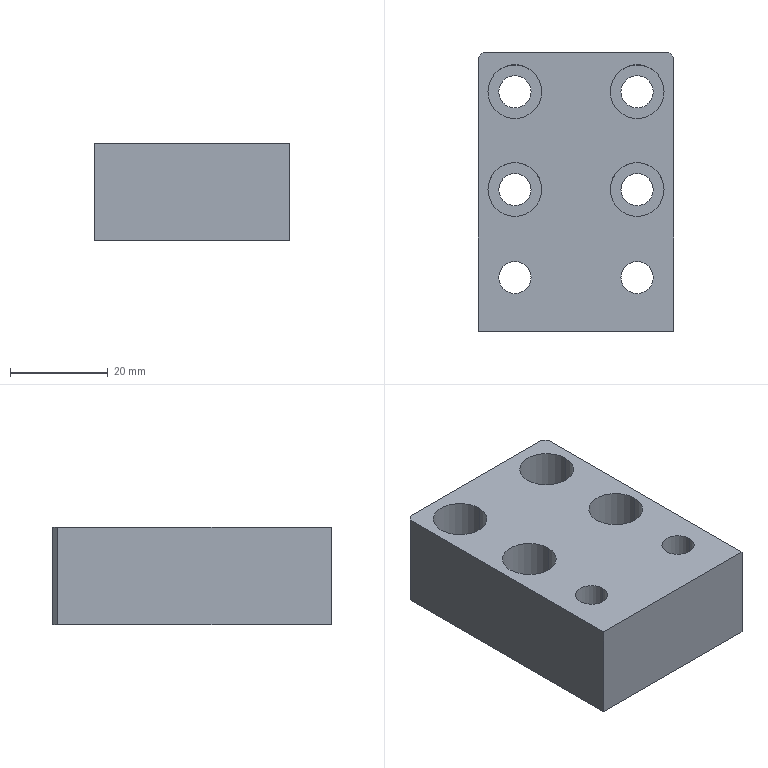Part | SolidWorks | features BaseBody 1 | 1 solid | 38 faces | box 40 x 57 x 20 mm | volume 37168 mm3 | cylinder 24 | plane 14 | commonest cylinder face diameters 6.6 x12 11 x12
STEP:
#1=CARTESIAN_POINT('',(-7.,-17.5,11.8));
#2=VERTEX_POINT('',#1);
#3=CARTESIAN_POINT('',(-18.,-17.5,11.8));
#4=VERTEX_POINT('',#3);
#5=CARTESIAN_POINT('',(-12.5,-17.5,11.8));
#6=DIRECTION('',(0.,0.,-1.));
#7=DIRECTION('',(-1.,0.,0.));
#8=AXIS2_PLACEMENT_3D('',#5,#6,#7);
#9=CIRCLE('',#8,5.5);
#10=EDGE_CURVE('',#2,#4,#9,.T.);
#11=ORIENTED_EDGE('',*,*,#10,.F.);
#12=CARTESIAN_POINT('',(-7.,-17.5,0.));
#13=VERTEX_POINT('',#12);
#14=CARTESIAN_POINT('',(-7.,-17.5,0.));
#15=DIRECTION('',(0.,0.,-1.));
#16=VECTOR('',#15,1000.);
#17=LINE('',#14,#16);
#18=EDGE_CURVE('',#2,#13,#17,.T.);
#19=ORIENTED_EDGE('',*,*,#18,.T.);
#20=CARTESIAN_POINT('',(-18.,-17.5,0.));
#21=VERTEX_POINT('',#20);
#22=CARTESIAN_POINT('',(-12.5,-17.5,0.));
#23=DIRECTION('',(0.,0.,-1.));
#24=DIRECTION('',(-1.,0.,0.));
#25=AXIS2_PLACEMENT_3D('',#22,#23,#24);
#26=CIRCLE('',#25,5.5);
#27=EDGE_CURVE('',#13,#21,#26,.T.);
#28=ORIENTED_EDGE('',*,*,#27,.T.);
#29=CARTESIAN_POINT('',(-18.,-17.5,0.));
#30=DIRECTION('',(0.,0.,-1.));
#31=VECTOR('',#30,1000.);
#32=LINE('',#29,#31);
#33=EDGE_CURVE('',#4,#21,#32,.T.);
#34=ORIENTED_EDGE('',*,*,#33,.F.);
#35=EDGE_LOOP('',(#11,#19,#28,#34));
#36=FACE_OUTER_BOUND('',#35,.T.);
#37=CARTESIAN_POINT('',(-12.5,-17.5,0.));
#38=DIRECTION('',(0.,0.,-1.));
#39=DIRECTION('',(-1.,0.,0.));
#40=AXIS2_PLACEMENT_3D('',#37,#38,#39);
#41=CYLINDRICAL_SURFACE('',#40,5.5);
#42=ADVANCED_FACE('',(#36),#41,.F.);
#43=CARTESIAN_POINT('',(-9.2,-17.5,20.));
#44=VERTEX_POINT('',#43);
#45=CARTESIAN_POINT('',(-15.8,-17.5,20.));
#46=VERTEX_POINT('',#45);
#47=CARTESIAN_POINT('',(-12.5,-17.5,20.));
#48=DIRECTION('',(0.,0.,-1.));
#49=DIRECTION('',(-1.,0.,0.));
#50=AXIS2_PLACEMENT_3D('',#47,#48,#49);
#51=CIRCLE('',#50,3.3);
#52=EDGE_CURVE('',#44,#46,#51,.T.);
#53=ORIENTED_EDGE('',*,*,#52,.F.);
#54=CARTESIAN_POINT('',(-9.2,-17.5,11.8));
#55=VERTEX_POINT('',#54);
#56=CARTESIAN_POINT('',(-9.2,-17.5,0.));
#57=DIRECTION('',(0.,0.,-1.));
#58=VECTOR('',#57,1000.);
#59=LINE('',#56,#58);
#60=EDGE_CURVE('',#44,#55,#59,.T.);
#61=ORIENTED_EDGE('',*,*,#60,.T.);
#62=CARTESIAN_POINT('',(-15.8,-17.5,11.8));
#63=VERTEX_POINT('',#62);
#64=CARTESIAN_POINT('',(-12.5,-17.5,11.8));
#65=DIRECTION('',(0.,0.,-1.));
#66=DIRECTION('',(-1.,0.,0.));
#67=AXIS2_PLACEMENT_3D('',#64,#65,#66);
#68=CIRCLE('',#67,3.3);
#69=EDGE_CURVE('',#55,#63,#68,.T.);
#70=ORIENTED_EDGE('',*,*,#69,.T.);
#71=CARTESIAN_POINT('',(-15.8,-17.5,0.));
#72=DIRECTION('',(0.,0.,-1.));
#73=VECTOR('',#72,1000.);
#74=LINE('',#71,#73);
#75=EDGE_CURVE('',#46,#63,#74,.T.);
#76=ORIENTED_EDGE('',*,*,#75,.F.);
#77=EDGE_LOOP('',(#53,#61,#70,#76));
#78=FACE_OUTER_BOUND('',#77,.T.);
#79=CARTESIAN_POINT('',(-12.5,-17.5,0.));
#80=DIRECTION('',(0.,0.,-1.));
#81=DIRECTION('',(-1.,0.,0.));
#82=AXIS2_PLACEMENT_3D('',#79,#80,#81);
#83=CYLINDRICAL_SURFACE('',#82,3.3);
#84=ADVANCED_FACE('',(#78),#83,.F.);
#85=CARTESIAN_POINT('',(18.,-17.5,11.8));
#86=VERTEX_POINT('',#85);
#87=CARTESIAN_POINT('',(7.,-17.5,11.8));
#88=VERTEX_POINT('',#87);
#89=CARTESIAN_POINT('',(12.5,-17.5,11.8));
#90=DIRECTION('',(0.,0.,-1.));
#91=DIRECTION('',(-1.,0.,0.));
#92=AXIS2_PLACEMENT_3D('',#89,#90,#91);
#93=CIRCLE('',#92,5.5);
#94=EDGE_CURVE('',#86,#88,#93,.T.);
#95=ORIENTED_EDGE('',*,*,#94,.F.);
#96=CARTESIAN_POINT('',(18.,-17.5,0.));
#97=VERTEX_POINT('',#96);
#98=CARTESIAN_POINT('',(18.,-17.5,0.));
#99=DIRECTION('',(0.,0.,-1.));
#100=VECTOR('',#99,1000.);
#101=LINE('',#98,#100);
#102=EDGE_CURVE('',#86,#97,#101,.T.);
#103=ORIENTED_EDGE('',*,*,#102,.T.);
#104=CARTESIAN_POINT('',(7.,-17.5,0.));
#105=VERTEX_POINT('',#104);
#106=CARTESIAN_POINT('',(12.5,-17.5,0.));
#107=DIRECTION('',(0.,0.,-1.));
#108=DIRECTION('',(-1.,0.,0.));
#109=AXIS2_PLACEMENT_3D('',#106,#107,#108);
#110=CIRCLE('',#109,5.5);
#111=EDGE_CURVE('',#97,#105,#110,.T.);
#112=ORIENTED_EDGE('',*,*,#111,.T.);
#113=CARTESIAN_POINT('',(7.,-17.5,0.));
#114=DIRECTION('',(0.,0.,-1.));
#115=VECTOR('',#114,1000.);
#116=LINE('',#113,#115);
#117=EDGE_CURVE('',#88,#105,#116,.T.);
#118=ORIENTED_EDGE('',*,*,#117,.F.);
#119=EDGE_LOOP('',(#95,#103,#112,#118));
#120=FACE_OUTER_BOUND('',#119,.T.);
#121=CARTESIAN_POINT('',(12.5,-17.5,0.));
#122=DIRECTION('',(0.,0.,-1.));
#123=DIRECTION('',(-1.,0.,0.));
#124=AXIS2_PLACEMENT_3D('',#121,#122,#123);
#125=CYLINDRICAL_SURFACE('',#124,5.5);
#126=ADVANCED_FACE('',(#120),#125,.F.);
#127=CARTESIAN_POINT('',(15.8,-17.5,20.));
#128=VERTEX_POINT('',#127);
#129=CARTESIAN_POINT('',(9.2,-17.5,20.));
#130=VERTEX_POINT('',#129);
#131=CARTESIAN_POINT('',(12.5,-17.5,20.));
#132=DIRECTION('',(0.,0.,-1.));
#133=DIRECTION('',(-1.,0.,0.));
#134=AXIS2_PLACEMENT_3D('',#131,#132,#133);
#135=CIRCLE('',#134,3.3);
#136=EDGE_CURVE('',#128,#130,#135,.T.);
#137=ORIENTED_EDGE('',*,*,#136,.F.);
#138=CARTESIAN_POINT('',(15.8,-17.5,11.8));
#139=VERTEX_POINT('',#138);
#140=CARTESIAN_POINT('',(15.8,-17.5,0.));
#141=DIRECTION('',(0.,0.,-1.));
#142=VECTOR('',#141,1000.);
#143=LINE('',#140,#142);
#144=EDGE_CURVE('',#128,#139,#143,.T.);
#145=ORIENTED_EDGE('',*,*,#144,.T.);
#146=CARTESIAN_POINT('',(9.2,-17.5,11.8));
#147=VERTEX_POINT('',#146);
#148=CARTESIAN_POINT('',(12.5,-17.5,11.8));
#149=DIRECTION('',(0.,0.,-1.));
#150=DIRECTION('',(-1.,0.,0.));
#151=AXIS2_PLACEMENT_3D('',#148,#149,#150);
#152=CIRCLE('',#151,3.3);
#153=EDGE_CURVE('',#139,#147,#152,.T.);
#154=ORIENTED_EDGE('',*,*,#153,.T.);
#155=CARTESIAN_POINT('',(9.2,-17.5,0.));
#156=DIRECTION('',(0.,0.,-1.));
#157=VECTOR('',#156,1000.);
#158=LINE('',#155,#157);
#159=EDGE_CURVE('',#130,#147,#158,.T.);
#160=ORIENTED_EDGE('',*,*,#159,.F.);
#161=EDGE_LOOP('',(#137,#145,#154,#160));
#162=FACE_OUTER_BOUND('',#161,.T.);
#163=CARTESIAN_POINT('',(12.5,-17.5,0.));
#164=DIRECTION('',(0.,0.,-1.));
#165=DIRECTION('',(-1.,0.,0.));
#166=AXIS2_PLACEMENT_3D('',#163,#164,#165);
#167=CYLINDRICAL_SURFACE('',#166,3.3);
#168=ADVANCED_FACE('',(#162),#167,.F.);
#169=CARTESIAN_POINT('',(7.,20.5,8.2));
#170=VERTEX_POINT('',#169);
#171=CARTESIAN_POINT('',(18.,20.5,8.2));
#172=VERTEX_POINT('',#171);
#173=CARTESIAN_POINT('',(12.5,20.5,8.2));
#174=DIRECTION('',(0.,0.,1.));
#175=DIRECTION('',(1.,0.,0.));
#176=AXIS2_PLACEMENT_3D('',#173,#174,#175);
#177=CIRCLE('',#176,5.5);
#178=EDGE_CURVE('',#170,#172,#177,.T.);
#179=ORIENTED_EDGE('',*,*,#178,.F.);
#180=CARTESIAN_POINT('',(7.,20.5,20.));
#181=VERTEX_POINT('',#180);
#182=CARTESIAN_POINT('',(7.,20.5,20.));
#183=DIRECTION('',(0.,0.,1.));
#184=VECTOR('',#183,1000.);
#185=LINE('',#182,#184);
#186=EDGE_CURVE('',#170,#181,#185,.T.);
#187=ORIENTED_EDGE('',*,*,#186,.T.);
#188=CARTESIAN_POINT('',(18.,20.5,20.));
#189=VERTEX_POINT('',#188);
#190=CARTESIAN_POINT('',(12.5,20.5,20.));
#191=DIRECTION('',(0.,0.,1.));
#192=DIRECTION('',(1.,0.,0.));
#193=AXIS2_PLACEMENT_3D('',#190,#191,#192);
#194=CIRCLE('',#193,5.5);
#195=EDGE_CURVE('',#181,#189,#194,.T.);
#196=ORIENTED_EDGE('',*,*,#195,.T.);
#197=CARTESIAN_POINT('',(18.,20.5,20.));
#198=DIRECTION('',(0.,0.,1.));
#199=VECTOR('',#198,1000.);
#200=LINE('',#197,#199);
#201=EDGE_CURVE('',#172,#189,#200,.T.);
#202=ORIENTED_EDGE('',*,*,#201,.F.);
#203=EDGE_LOOP('',(#179,#187,#196,#202));
#204=FACE_OUTER_BOUND('',#203,.T.);
#205=CARTESIAN_POINT('',(12.5,20.5,20.));
#206=DIRECTION('',(0.,0.,1.));
#207=DIRECTION('',(1.,0.,0.));
#208=AXIS2_PLACEMENT_3D('',#205,#206,#207);
#209=CYLINDRICAL_SURFACE('',#208,5.5);
#210=ADVANCED_FACE('',(#204),#209,.F.);
#211=CARTESIAN_POINT('',(15.8,20.5,0.));
#212=VERTEX_POINT('',#211);
#213=CARTESIAN_POINT('',(9.2,20.5,0.));
#214=VERTEX_POINT('',#213);
#215=CARTESIAN_POINT('',(12.5,20.5,0.));
#216=DIRECTION('',(0.,0.,-1.));
#217=DIRECTION('',(-1.,0.,0.));
#218=AXIS2_PLACEMENT_3D('',#215,#216,#217);
#219=CIRCLE('',#218,3.3);
#220=EDGE_CURVE('',#212,#214,#219,.T.);
#221=ORIENTED_EDGE('',*,*,#220,.T.);
#222=CARTESIAN_POINT('',(9.2,20.5,8.2));
#223=VERTEX_POINT('',#222);
#224=CARTESIAN_POINT('',(9.2,20.5,20.));
#225=DIRECTION('',(0.,0.,1.));
#226=VECTOR('',#225,1000.);
#227=LINE('',#224,#226);
#228=EDGE_CURVE('',#214,#223,#227,.T.);
#229=ORIENTED_EDGE('',*,*,#228,.T.);
#230=CARTESIAN_POINT('',(15.8,20.5,8.2));
#231=VERTEX_POINT('',#230);
#232=CARTESIAN_POINT('',(12.5,20.5,8.2));
#233=DIRECTION('',(0.,0.,1.));
#234=DIRECTION('',(1.,0.,0.));
#235=AXIS2_PLACEMENT_3D('',#232,#233,#234);
#236=CIRCLE('',#235,3.3);
#237=EDGE_CURVE('',#223,#231,#236,.T.);
#238=ORIENTED_EDGE('',*,*,#237,.T.);
#239=CARTESIAN_POINT('',(15.8,20.5,20.));
#240=DIRECTION('',(0.,0.,1.));
#241=VECTOR('',#240,1000.);
#242=LINE('',#239,#241);
#243=EDGE_CURVE('',#212,#231,#242,.T.);
#244=ORIENTED_EDGE('',*,*,#243,.F.);
#245=EDGE_LOOP('',(#221,#229,#238,#244));
#246=FACE_OUTER_BOUND('',#245,.T.);
#247=CARTESIAN_POINT('',(12.5,20.5,20.));
#248=DIRECTION('',(0.,0.,1.));
#249=DIRECTION('',(1.,0.,0.));
#250=AXIS2_PLACEMENT_3D('',#247,#248,#249);
#251=CYLINDRICAL_SURFACE('',#250,3.3);
#252=ADVANCED_FACE('',(#246),#251,.F.);
#253=CARTESIAN_POINT('',(-18.,20.5,8.2));
#254=VERTEX_POINT('',#253);
#255=CARTESIAN_POINT('',(-7.,20.5,8.2));
#256=VERTEX_POINT('',#255);
#257=CARTESIAN_POINT('',(-12.5,20.5,8.2));
#258=DIRECTION('',(0.,0.,1.));
#259=DIRECTION('',(1.,0.,0.));
#260=AXIS2_PLACEMENT_3D('',#257,#258,#259);
#261=CIRCLE('',#260,5.5);
#262=EDGE_CURVE('',#254,#256,#261,.T.);
#263=ORIENTED_EDGE('',*,*,#262,.F.);
#264=CARTESIAN_POINT('',(-18.,20.5,20.));
#265=VERTEX_POINT('',#264);
#266=CARTESIAN_POINT('',(-18.,20.5,20.));
#267=DIRECTION('',(0.,0.,1.));
#268=VECTOR('',#267,1000.);
#269=LINE('',#266,#268);
#270=EDGE_CURVE('',#254,#265,#269,.T.);
#271=ORIENTED_EDGE('',*,*,#270,.T.);
#272=CARTESIAN_POINT('',(-7.,20.5,20.));
#273=VERTEX_POINT('',#272);
#274=CARTESIAN_POINT('',(-12.5,20.5,20.));
#275=DIRECTION('',(0.,0.,1.));
#276=DIRECTION('',(1.,0.,0.));
#277=AXIS2_PLACEMENT_3D('',#274,#275,#276);
#278=CIRCLE('',#277,5.5);
#279=EDGE_CURVE('',#265,#273,#278,.T.);
#280=ORIENTED_EDGE('',*,*,#279,.T.);
#281=CARTESIAN_POINT('',(-7.,20.5,20.));
#282=DIRECTION('',(0.,0.,1.));
#283=VECTOR('',#282,1000.);
#284=LINE('',#281,#283);
#285=EDGE_CURVE('',#256,#273,#284,.T.);
#286=ORIENTED_EDGE('',*,*,#285,.F.);
#287=EDGE_LOOP('',(#263,#271,#280,#286));
#288=FACE_OUTER_BOUND('',#287,.T.);
#289=CARTESIAN_POINT('',(-12.5,20.5,20.));
#290=DIRECTION('',(0.,0.,1.));
#291=DIRECTION('',(1.,0.,0.));
#292=AXIS2_PLACEMENT_3D('',#289,#290,#291);
#293=CYLINDRICAL_SURFACE('',#292,5.5);
#294=ADVANCED_FACE('',(#288),#293,.F.);
#295=CARTESIAN_POINT('',(-9.2,20.5,0.));
#296=VERTEX_POINT('',#295);
#297=CARTESIAN_POINT('',(-15.8,20.5,0.));
#298=VERTEX_POINT('',#297);
#299=CARTESIAN_POINT('',(-12.5,20.5,0.));
#300=DIRECTION('',(0.,0.,-1.));
#301=DIRECTION('',(-1.,0.,0.));
#302=AXIS2_PLACEMENT_3D('',#299,#300,#301);
#303=CIRCLE('',#302,3.3);
#304=EDGE_CURVE('',#296,#298,#303,.T.);
#305=ORIENTED_EDGE('',*,*,#304,.T.);
#306=CARTESIAN_POINT('',(-15.8,20.5,8.2));
#307=VERTEX_POINT('',#306);
#308=CARTESIAN_POINT('',(-15.8,20.5,20.));
#309=DIRECTION('',(0.,0.,1.));
#310=VECTOR('',#309,1000.);
#311=LINE('',#308,#310);
#312=EDGE_CURVE('',#298,#307,#311,.T.);
#313=ORIENTED_EDGE('',*,*,#312,.T.);
#314=CARTESIAN_POINT('',(-9.2,20.5,8.2));
#315=VERTEX_POINT('',#314);
#316=CARTESIAN_POINT('',(-12.5,20.5,8.2));
#317=DIRECTION('',(0.,0.,1.));
#318=DIRECTION('',(1.,0.,0.));
#319=AXIS2_PLACEMENT_3D('',#316,#317,#318);
#320=CIRCLE('',#319,3.3);
#321=EDGE_CURVE('',#307,#315,#320,.T.);
#322=ORIENTED_EDGE('',*,*,#321,.T.);
#323=CARTESIAN_POINT('',(-9.2,20.5,20.));
#324=DIRECTION('',(0.,0.,1.));
#325=VECTOR('',#324,1000.);
#326=LINE('',#323,#325);
#327=EDGE_CURVE('',#296,#315,#326,.T.);
#328=ORIENTED_EDGE('',*,*,#327,.F.);
#329=EDGE_LOOP('',(#305,#313,#322,#328));
#330=FACE_OUTER_BOUND('',#329,.T.);
#331=CARTESIAN_POINT('',(-12.5,20.5,20.));
#332=DIRECTION('',(0.,0.,1.));
#333=DIRECTION('',(1.,0.,0.));
#334=AXIS2_PLACEMENT_3D('',#331,#332,#333);
#335=CYLINDRICAL_SURFACE('',#334,3.3);
#336=ADVANCED_FACE('',(#330),#335,.F.);
#337=CARTESIAN_POINT('',(7.,0.5,8.2));
#338=VERTEX_POINT('',#337);
#339=CARTESIAN_POINT('',(18.,0.5,8.2));
#340=VERTEX_POINT('',#339);
#341=CARTESIAN_POINT('',(12.5,0.5,8.2));
#342=DIRECTION('',(0.,0.,1.));
#343=DIRECTION('',(1.,0.,0.));
#344=AXIS2_PLACEMENT_3D('',#341,#342,#343);
#345=CIRCLE('',#344,5.5);
#346=EDGE_CURVE('',#338,#340,#345,.T.);
#347=ORIENTED_EDGE('',*,*,#346,.F.);
#348=CARTESIAN_POINT('',(7.,0.5,20.));
#349=VERTEX_POINT('',#348);
#350=CARTESIAN_POINT('',(7.,0.5,20.));
#351=DIRECTION('',(0.,0.,1.));
#352=VECTOR('',#351,1000.);
#353=LINE('',#350,#352);
#354=EDGE_CURVE('',#338,#349,#353,.T.);
#355=ORIENTED_EDGE('',*,*,#354,.T.);
#356=CARTESIAN_POINT('',(18.,0.5,20.));
#357=VERTEX_POINT('',#356);
#358=CARTESIAN_POINT('',(12.5,0.5,20.));
#359=DIRECTION('',(0.,0.,1.));
#360=DIRECTION('',(1.,0.,0.));
#361=AXIS2_PLACEMENT_3D('',#358,#359,#360);
#362=CIRCLE('',#361,5.5);
#363=EDGE_CURVE('',#349,#357,#362,.T.);
#364=ORIENTED_EDGE('',*,*,#363,.T.);
#365=CARTESIAN_POINT('',(18.,0.5,20.));
#366=DIRECTION('',(0.,0.,1.));
#367=VECTOR('',#366,1000.);
#368=LINE('',#365,#367);
#369=EDGE_CURVE('',#340,#357,#368,.T.);
#370=ORIENTED_EDGE('',*,*,#369,.F.);
#371=EDGE_LOOP('',(#347,#355,#364,#370));
#372=FACE_OUTER_BOUND('',#371,.T.);
#373=CARTESIAN_POINT('',(12.5,0.5,20.));
#374=DIRECTION('',(0.,0.,1.));
#375=DIRECTION('',(1.,0.,0.));
#376=AXIS2_PLACEMENT_3D('',#373,#374,#375);
#377=CYLINDRICAL_SURFACE('',#376,5.5);
#378=ADVANCED_FACE('',(#372),#377,.F.);
#379=CARTESIAN_POINT('',(15.8,0.5,0.));
#380=VERTEX_POINT('',#379);
#381=CARTESIAN_POINT('',(9.2,0.5,0.));
#382=VERTEX_POINT('',#381);
#383=CARTESIAN_POINT('',(12.5,0.5,0.));
#384=DIRECTION('',(0.,0.,-1.));
#385=DIRECTION('',(-1.,0.,0.));
#386=AXIS2_PLACEMENT_3D('',#383,#384,#385);
#387=CIRCLE('',#386,3.3);
#388=EDGE_CURVE('',#380,#382,#387,.T.);
#389=ORIENTED_EDGE('',*,*,#388,.T.);
#390=CARTESIAN_POINT('',(9.2,0.5,8.2));
#391=VERTEX_POINT('',#390);
#392=CARTESIAN_POINT('',(9.2,0.5,20.));
#393=DIRECTION('',(0.,0.,1.));
#394=VECTOR('',#393,1000.);
#395=LINE('',#392,#394);
#396=EDGE_CURVE('',#382,#391,#395,.T.);
#397=ORIENTED_EDGE('',*,*,#396,.T.);
#398=CARTESIAN_POINT('',(15.8,0.5,8.2));
#399=VERTEX_POINT('',#398);
#400=CARTESIAN_POINT('',(12.5,0.5,8.2));
#401=DIRECTION('',(0.,0.,1.));
#402=DIRECTION('',(1.,0.,0.));
#403=AXIS2_PLACEMENT_3D('',#400,#401,#402);
#404=CIRCLE('',#403,3.3);
#405=EDGE_CURVE('',#391,#399,#404,.T.);
#406=ORIENTED_EDGE('',*,*,#405,.T.);
#407=CARTESIAN_POINT('',(15.8,0.5,20.));
#408=DIRECTION('',(0.,0.,1.));
#409=VECTOR('',#408,1000.);
#410=LINE('',#407,#409);
#411=EDGE_CURVE('',#380,#399,#410,.T.);
#412=ORIENTED_EDGE('',*,*,#411,.F.);
#413=EDGE_LOOP('',(#389,#397,#406,#412));
#414=FACE_OUTER_BOUND('',#413,.T.);
#415=CARTESIAN_POINT('',(12.5,0.5,20.));
#416=DIRECTION('',(0.,0.,1.));
#417=DIRECTION('',(1.,0.,0.));
#418=AXIS2_PLACEMENT_3D('',#415,#416,#417);
#419=CYLINDRICAL_SURFACE('',#418,3.3);
#420=ADVANCED_FACE('',(#414),#419,.F.);
#421=CARTESIAN_POINT('',(-18.,0.5,8.2));
#422=VERTEX_POINT('',#421);
#423=CARTESIAN_POINT('',(-7.,0.5,8.2));
#424=VERTEX_POINT('',#423);
#425=CARTESIAN_POINT('',(-12.5,0.5,8.2));
#426=DIRECTION('',(0.,0.,1.));
#427=DIRECTION('',(1.,0.,0.));
#428=AXIS2_PLACEMENT_3D('',#425,#426,#427);
#429=CIRCLE('',#428,5.5);
#430=EDGE_CURVE('',#422,#424,#429,.T.);
#431=ORIENTED_EDGE('',*,*,#430,.F.);
#432=CARTESIAN_POINT('',(-18.,0.5,20.));
#433=VERTEX_POINT('',#432);
#434=CARTESIAN_POINT('',(-18.,0.5,20.));
#435=DIRECTION('',(0.,0.,1.));
#436=VECTOR('',#435,1000.);
#437=LINE('',#434,#436);
#438=EDGE_CURVE('',#422,#433,#437,.T.);
#439=ORIENTED_EDGE('',*,*,#438,.T.);
#440=CARTESIAN_POINT('',(-7.,0.5,20.));
#441=VERTEX_POINT('',#440);
#442=CARTESIAN_POINT('',(-12.5,0.5,20.));
#443=DIRECTION('',(0.,0.,1.));
#444=DIRECTION('',(1.,0.,0.));
#445=AXIS2_PLACEMENT_3D('',#442,#443,#444);
#446=CIRCLE('',#445,5.5);
#447=EDGE_CURVE('',#433,#441,#446,.T.);
#448=ORIENTED_EDGE('',*,*,#447,.T.);
#449=CARTESIAN_POINT('',(-7.,0.5,20.));
#450=DIRECTION('',(0.,0.,1.));
#451=VECTOR('',#450,1000.);
#452=LINE('',#449,#451);
#453=EDGE_CURVE('',#424,#441,#452,.T.);
#454=ORIENTED_EDGE('',*,*,#453,.F.);
#455=EDGE_LOOP('',(#431,#439,#448,#454));
#456=FACE_OUTER_BOUND('',#455,.T.);
#457=CARTESIAN_POINT('',(-12.5,0.5,20.));
#458=DIRECTION('',(0.,0.,1.));
#459=DIRECTION('',(1.,0.,0.));
#460=AXIS2_PLACEMENT_3D('',#457,#458,#459);
#461=CYLINDRICAL_SURFACE('',#460,5.5);
#462=ADVANCED_FACE('',(#456),#461,.F.);
#463=CARTESIAN_POINT('',(-9.2,0.5,0.));
#464=VERTEX_POINT('',#463);
#465=CARTESIAN_POINT('',(-15.8,0.5,0.));
#466=VERTEX_POINT('',#465);
#467=CARTESIAN_POINT('',(-12.5,0.5,0.));
#468=DIRECTION('',(0.,0.,-1.));
#469=DIRECTION('',(-1.,0.,0.));
#470=AXIS2_PLACEMENT_3D('',#467,#468,#469);
#471=CIRCLE('',#470,3.3);
#472=EDGE_CURVE('',#464,#466,#471,.T.);
#473=ORIENTED_EDGE('',*,*,#472,.T.);
#474=CARTESIAN_POINT('',(-15.8,0.5,8.2));
#475=VERTEX_POINT('',#474);
#476=CARTESIAN_POINT('',(-15.8,0.5,20.));
#477=DIRECTION('',(0.,0.,1.));
#478=VECTOR('',#477,1000.);
#479=LINE('',#476,#478);
#480=EDGE_CURVE('',#466,#475,#479,.T.);
#481=ORIENTED_EDGE('',*,*,#480,.T.);
#482=CARTESIAN_POINT('',(-9.2,0.5,8.2));
#483=VERTEX_POINT('',#482);
#484=CARTESIAN_POINT('',(-12.5,0.5,8.2));
#485=DIRECTION('',(0.,0.,1.));
#486=DIRECTION('',(1.,0.,0.));
#487=AXIS2_PLACEMENT_3D('',#484,#485,#486);
#488=CIRCLE('',#487,3.3);
#489=EDGE_CURVE('',#475,#483,#488,.T.);
#490=ORIENTED_EDGE('',*,*,#489,.T.);
#491=CARTESIAN_POINT('',(-9.2,0.5,20.));
#492=DIRECTION('',(0.,0.,1.));
#493=VECTOR('',#492,1000.);
#494=LINE('',#491,#493);
#495=EDGE_CURVE('',#464,#483,#494,.T.);
#496=ORIENTED_EDGE('',*,*,#495,.F.);
#497=EDGE_LOOP('',(#473,#481,#490,#496));
#498=FACE_OUTER_BOUND('',#497,.T.);
#499=CARTESIAN_POINT('',(-12.5,0.5,20.));
#500=DIRECTION('',(0.,0.,1.));
#501=DIRECTION('',(1.,0.,0.));
#502=AXIS2_PLACEMENT_3D('',#499,#500,#501);
#503=CYLINDRICAL_SURFACE('',#502,3.3);
#504=ADVANCED_FACE('',(#498),#503,.F.);
#505=CARTESIAN_POINT('',(20.,27.5,20.));
#506=VERTEX_POINT('',#505);
#507=CARTESIAN_POINT('',(19.,28.5,20.));
#508=VERTEX_POINT('',#507);
#509=CARTESIAN_POINT('',(19.,28.5,20.));
#510=DIRECTION('',(-0.7071,0.7071,0.));
#511=VECTOR('',#510,1000.);
#512=LINE('',#509,#511);
#513=EDGE_CURVE('',#506,#508,#512,.T.);
#514=ORIENTED_EDGE('',*,*,#513,.F.);
#515=CARTESIAN_POINT('',(20.,27.5,0.));
#516=VERTEX_POINT('',#515);
#517=CARTESIAN_POINT('',(20.,27.5,20.));
#518=DIRECTION('',(0.,0.,1.));
#519=VECTOR('',#518,1000.);
#520=LINE('',#517,#519);
#521=EDGE_CURVE('',#516,#506,#520,.T.);
#522=ORIENTED_EDGE('',*,*,#521,.F.);
#523=CARTESIAN_POINT('',(19.,28.5,0.));
#524=VERTEX_POINT('',#523);
#525=CARTESIAN_POINT('',(23.75,23.75,0.));
#526=DIRECTION('',(0.7071,-0.7071,0.));
#527=VECTOR('',#526,1000.);
#528=LINE('',#525,#527);
#529=EDGE_CURVE('',#524,#516,#528,.T.);
#530=ORIENTED_EDGE('',*,*,#529,.F.);
#531=CARTESIAN_POINT('',(19.,28.5,20.));
#532=DIRECTION('',(0.,0.,-1.));
#533=VECTOR('',#532,1000.);
#534=LINE('',#531,#533);
#535=EDGE_CURVE('',#508,#524,#534,.T.);
#536=ORIENTED_EDGE('',*,*,#535,.F.);
#537=EDGE_LOOP('',(#514,#522,#530,#536));
#538=FACE_OUTER_BOUND('',#537,.T.);
#539=CARTESIAN_POINT('',(19.,28.5,20.));
#540=DIRECTION('',(-0.7071,-0.7071,0.));
#541=DIRECTION('',(-0.7071,0.7071,0.));
#542=AXIS2_PLACEMENT_3D('',#539,#540,#541);
#543=PLANE('',#542);
#544=ADVANCED_FACE('',(#538),#543,.F.);
#545=CARTESIAN_POINT('',(-19.,28.5,20.));
#546=VERTEX_POINT('',#545);
#547=CARTESIAN_POINT('',(-20.,27.5,20.));
#548=VERTEX_POINT('',#547);
#549=CARTESIAN_POINT('',(-20.,27.5,20.));
#550=DIRECTION('',(-0.7071,-0.7071,0.));
#551=VECTOR('',#550,1000.);
#552=LINE('',#549,#551);
#553=EDGE_CURVE('',#546,#548,#552,.T.);
#554=ORIENTED_EDGE('',*,*,#553,.F.);
#555=CARTESIAN_POINT('',(-19.,28.5,0.));
#556=VERTEX_POINT('',#555);
#557=CARTESIAN_POINT('',(-19.,28.5,20.));
#558=DIRECTION('',(0.,0.,1.));
#559=VECTOR('',#558,1000.);
#560=LINE('',#557,#559);
#561=EDGE_CURVE('',#556,#546,#560,.T.);
#562=ORIENTED_EDGE('',*,*,#561,.F.);
#563=CARTESIAN_POINT('',(-20.,27.5,0.));
#564=VERTEX_POINT('',#563);
#565=CARTESIAN_POINT('',(-23.75,23.75,0.));
#566=DIRECTION('',(0.7071,0.7071,0.));
#567=VECTOR('',#566,1000.);
#568=LINE('',#565,#567);
#569=EDGE_CURVE('',#564,#556,#568,.T.);
#570=ORIENTED_EDGE('',*,*,#569,.F.);
#571=CARTESIAN_POINT('',(-20.,27.5,20.));
#572=DIRECTION('',(0.,0.,-1.));
#573=VECTOR('',#572,1000.);
#574=LINE('',#571,#573);
#575=EDGE_CURVE('',#548,#564,#574,.T.);
#576=ORIENTED_EDGE('',*,*,#575,.F.);
#577=EDGE_LOOP('',(#554,#562,#570,#576));
#578=FACE_OUTER_BOUND('',#577,.T.);
#579=CARTESIAN_POINT('',(-20.,27.5,20.));
#580=DIRECTION('',(0.7071,-0.7071,0.));
#581=DIRECTION('',(0.,0.,-1.));
#582=AXIS2_PLACEMENT_3D('',#579,#580,#581);
#583=PLANE('',#582);
#584=ADVANCED_FACE('',(#578),#583,.F.);
#585=CARTESIAN_POINT('',(-12.5,-17.5,11.8));
#586=DIRECTION('',(0.,0.,-1.));
#587=DIRECTION('',(-1.,0.,0.));
#588=AXIS2_PLACEMENT_3D('',#585,#586,#587);
#589=CIRCLE('',#588,3.3);
#590=EDGE_CURVE('',#63,#55,#589,.T.);
#591=ORIENTED_EDGE('',*,*,#590,.F.);
#592=ORIENTED_EDGE('',*,*,#69,.F.);
#593=EDGE_LOOP('',(#591,#592));
#594=FACE_BOUND('',#593,.T.);
#595=CARTESIAN_POINT('',(-12.5,-17.5,11.8));
#596=DIRECTION('',(0.,0.,-1.));
#597=DIRECTION('',(-1.,0.,0.));
#598=AXIS2_PLACEMENT_3D('',#595,#596,#597);
#599=CIRCLE('',#598,5.5);
#600=EDGE_CURVE('',#4,#2,#599,.T.);
#601=ORIENTED_EDGE('',*,*,#600,.T.);
#602=ORIENTED_EDGE('',*,*,#10,.T.);
#603=EDGE_LOOP('',(#601,#602));
#604=FACE_OUTER_BOUND('',#603,.T.);
#605=CARTESIAN_POINT('',(-9.2,-17.5,11.8));
#606=DIRECTION('',(0.,0.,1.));
#607=DIRECTION('',(1.,0.,0.));
#608=AXIS2_PLACEMENT_3D('',#605,#606,#607);
#609=PLANE('',#608);
#610=ADVANCED_FACE('',(#594,#604),#609,.F.);
#611=CARTESIAN_POINT('',(12.5,-17.5,11.8));
#612=DIRECTION('',(0.,0.,-1.));
#613=DIRECTION('',(-1.,0.,0.));
#614=AXIS2_PLACEMENT_3D('',#611,#612,#613);
#615=CIRCLE('',#614,3.3);
#616=EDGE_CURVE('',#147,#139,#615,.T.);
#617=ORIENTED_EDGE('',*,*,#616,.F.);
#618=ORIENTED_EDGE('',*,*,#153,.F.);
#619=EDGE_LOOP('',(#617,#618));
#620=FACE_BOUND('',#619,.T.);
#621=CARTESIAN_POINT('',(12.5,-17.5,11.8));
#622=DIRECTION('',(0.,0.,-1.));
#623=DIRECTION('',(-1.,0.,0.));
#624=AXIS2_PLACEMENT_3D('',#621,#622,#623);
#625=CIRCLE('',#624,5.5);
#626=EDGE_CURVE('',#88,#86,#625,.T.);
#627=ORIENTED_EDGE('',*,*,#626,.T.);
#628=ORIENTED_EDGE('',*,*,#94,.T.);
#629=EDGE_LOOP('',(#627,#628));
#630=FACE_OUTER_BOUND('',#629,.T.);
#631=CARTESIAN_POINT('',(15.8,-17.5,11.8));
#632=DIRECTION('',(0.,0.,1.));
#633=DIRECTION('',(1.,0.,0.));
#634=AXIS2_PLACEMENT_3D('',#631,#632,#633);
#635=PLANE('',#634);
#636=ADVANCED_FACE('',(#620,#630),#635,.F.);
#637=CARTESIAN_POINT('',(12.5,20.5,8.2));
#638=DIRECTION('',(0.,0.,1.));
#639=DIRECTION('',(1.,0.,0.));
#640=AXIS2_PLACEMENT_3D('',#637,#638,#639);
#641=CIRCLE('',#640,3.3);
#642=EDGE_CURVE('',#231,#223,#641,.T.);
#643=ORIENTED_EDGE('',*,*,#642,.F.);
#644=ORIENTED_EDGE('',*,*,#237,.F.);
#645=EDGE_LOOP('',(#643,#644));
#646=FACE_BOUND('',#645,.T.);
#647=CARTESIAN_POINT('',(12.5,20.5,8.2));
#648=DIRECTION('',(0.,0.,1.));
#649=DIRECTION('',(1.,0.,0.));
#650=AXIS2_PLACEMENT_3D('',#647,#648,#649);
#651=CIRCLE('',#650,5.5);
#652=EDGE_CURVE('',#172,#170,#651,.T.);
#653=ORIENTED_EDGE('',*,*,#652,.T.);
#654=ORIENTED_EDGE('',*,*,#178,.T.);
#655=EDGE_LOOP('',(#653,#654));
#656=FACE_OUTER_BOUND('',#655,.T.);
#657=CARTESIAN_POINT('',(15.8,20.5,8.2));
#658=DIRECTION('',(0.,0.,-1.));
#659=DIRECTION('',(0.,-1.,0.));
#660=AXIS2_PLACEMENT_3D('',#657,#658,#659);
#661=PLANE('',#660);
#662=ADVANCED_FACE('',(#646,#656),#661,.F.);
#663=CARTESIAN_POINT('',(-12.5,20.5,8.2));
#664=DIRECTION('',(0.,0.,1.));
#665=DIRECTION('',(1.,0.,0.));
#666=AXIS2_PLACEMENT_3D('',#663,#664,#665);
#667=CIRCLE('',#666,3.3);
#668=EDGE_CURVE('',#315,#307,#667,.T.);
#669=ORIENTED_EDGE('',*,*,#668,.F.);
#670=ORIENTED_EDGE('',*,*,#321,.F.);
#671=EDGE_LOOP('',(#669,#670));
#672=FACE_BOUND('',#671,.T.);
#673=CARTESIAN_POINT('',(-12.5,20.5,8.2));
#674=DIRECTION('',(0.,0.,1.));
#675=DIRECTION('',(1.,0.,0.));
#676=AXIS2_PLACEMENT_3D('',#673,#674,#675);
#677=CIRCLE('',#676,5.5);
#678=EDGE_CURVE('',#256,#254,#677,.T.);
#679=ORIENTED_EDGE('',*,*,#678,.T.);
#680=ORIENTED_EDGE('',*,*,#262,.T.);
#681=EDGE_LOOP('',(#679,#680));
#682=FACE_OUTER_BOUND('',#681,.T.);
#683=CARTESIAN_POINT('',(-9.2,20.5,8.2));
#684=DIRECTION('',(0.,0.,-1.));
#685=DIRECTION('',(0.,-1.,0.));
#686=AXIS2_PLACEMENT_3D('',#683,#684,#685);
#687=PLANE('',#686);
#688=ADVANCED_FACE('',(#672,#682),#687,.F.);
#689=CARTESIAN_POINT('',(12.5,0.5,8.2));
#690=DIRECTION('',(0.,0.,1.));
#691=DIRECTION('',(1.,0.,0.));
#692=AXIS2_PLACEMENT_3D('',#689,#690,#691);
#693=CIRCLE('',#692,3.3);
#694=EDGE_CURVE('',#399,#391,#693,.T.);
#695=ORIENTED_EDGE('',*,*,#694,.F.);
#696=ORIENTED_EDGE('',*,*,#405,.F.);
#697=EDGE_LOOP('',(#695,#696));
#698=FACE_BOUND('',#697,.T.);
#699=CARTESIAN_POINT('',(12.5,0.5,8.2));
#700=DIRECTION('',(0.,0.,1.));
#701=DIRECTION('',(1.,0.,0.));
#702=AXIS2_PLACEMENT_3D('',#699,#700,#701);
#703=CIRCLE('',#702,5.5);
#704=EDGE_CURVE('',#340,#338,#703,.T.);
#705=ORIENTED_EDGE('',*,*,#704,.T.);
#706=ORIENTED_EDGE('',*,*,#346,.T.);
#707=EDGE_LOOP('',(#705,#706));
#708=FACE_OUTER_BOUND('',#707,.T.);
#709=CARTESIAN_POINT('',(15.8,0.5,8.2));
#710=DIRECTION('',(0.,0.,-1.));
#711=DIRECTION('',(0.,-1.,0.));
#712=AXIS2_PLACEMENT_3D('',#709,#710,#711);
#713=PLANE('',#712);
#714=ADVANCED_FACE('',(#698,#708),#713,.F.);
#715=CARTESIAN_POINT('',(-12.5,0.5,8.2));
#716=DIRECTION('',(0.,0.,1.));
#717=DIRECTION('',(1.,0.,0.));
#718=AXIS2_PLACEMENT_3D('',#715,#716,#717);
#719=CIRCLE('',#718,3.3);
#720=EDGE_CURVE('',#483,#475,#719,.T.);
#721=ORIENTED_EDGE('',*,*,#720,.F.);
#722=ORIENTED_EDGE('',*,*,#489,.F.);
#723=EDGE_LOOP('',(#721,#722));
#724=FACE_BOUND('',#723,.T.);
#725=CARTESIAN_POINT('',(-12.5,0.5,8.2));
#726=DIRECTION('',(0.,0.,1.));
#727=DIRECTION('',(1.,0.,0.));
#728=AXIS2_PLACEMENT_3D('',#725,#726,#727);
#729=CIRCLE('',#728,5.5);
#730=EDGE_CURVE('',#424,#422,#729,.T.);
#731=ORIENTED_EDGE('',*,*,#730,.T.);
#732=ORIENTED_EDGE('',*,*,#430,.T.);
#733=EDGE_LOOP('',(#731,#732));
#734=FACE_OUTER_BOUND('',#733,.T.);
#735=CARTESIAN_POINT('',(-9.2,0.5,8.2));
#736=DIRECTION('',(0.,0.,-1.));
#737=DIRECTION('',(0.,-1.,0.));
#738=AXIS2_PLACEMENT_3D('',#735,#736,#737);
#739=PLANE('',#738);
#740=ADVANCED_FACE('',(#724,#734),#739,.F.);
#741=ORIENTED_EDGE('',*,*,#472,.F.);
#742=CARTESIAN_POINT('',(-12.5,0.5,0.));
#743=DIRECTION('',(0.,0.,-1.));
#744=DIRECTION('',(-1.,0.,0.));
#745=AXIS2_PLACEMENT_3D('',#742,#743,#744);
#746=CIRCLE('',#745,3.3);
#747=EDGE_CURVE('',#466,#464,#746,.T.);
#748=ORIENTED_EDGE('',*,*,#747,.F.);
#749=EDGE_LOOP('',(#741,#748));
#750=FACE_BOUND('',#749,.T.);
#751=ORIENTED_EDGE('',*,*,#388,.F.);
#752=CARTESIAN_POINT('',(12.5,0.5,0.));
#753=DIRECTION('',(0.,0.,-1.));
#754=DIRECTION('',(-1.,0.,0.));
#755=AXIS2_PLACEMENT_3D('',#752,#753,#754);
#756=CIRCLE('',#755,3.3);
#757=EDGE_CURVE('',#382,#380,#756,.T.);
#758=ORIENTED_EDGE('',*,*,#757,.F.);
#759=EDGE_LOOP('',(#751,#758));
#760=FACE_BOUND('',#759,.T.);
#761=ORIENTED_EDGE('',*,*,#304,.F.);
#762=CARTESIAN_POINT('',(-12.5,20.5,0.));
#763=DIRECTION('',(0.,0.,-1.));
#764=DIRECTION('',(-1.,0.,0.));
#765=AXIS2_PLACEMENT_3D('',#762,#763,#764);
#766=CIRCLE('',#765,3.3);
#767=EDGE_CURVE('',#298,#296,#766,.T.);
#768=ORIENTED_EDGE('',*,*,#767,.F.);
#769=EDGE_LOOP('',(#761,#768));
#770=FACE_BOUND('',#769,.T.);
#771=ORIENTED_EDGE('',*,*,#220,.F.);
#772=CARTESIAN_POINT('',(12.5,20.5,0.));
#773=DIRECTION('',(0.,0.,-1.));
#774=DIRECTION('',(-1.,0.,0.));
#775=AXIS2_PLACEMENT_3D('',#772,#773,#774);
#776=CIRCLE('',#775,3.3);
#777=EDGE_CURVE('',#214,#212,#776,.T.);
#778=ORIENTED_EDGE('',*,*,#777,.F.);
#779=EDGE_LOOP('',(#771,#778));
#780=FACE_BOUND('',#779,.T.);
#781=CARTESIAN_POINT('',(12.5,-17.5,0.));
#782=DIRECTION('',(0.,0.,-1.));
#783=DIRECTION('',(-1.,0.,0.));
#784=AXIS2_PLACEMENT_3D('',#781,#782,#783);
#785=CIRCLE('',#784,5.5);
#786=EDGE_CURVE('',#105,#97,#785,.T.);
#787=ORIENTED_EDGE('',*,*,#786,.F.);
#788=ORIENTED_EDGE('',*,*,#111,.F.);
#789=EDGE_LOOP('',(#787,#788));
#790=FACE_BOUND('',#789,.T.);
#791=CARTESIAN_POINT('',(-12.5,-17.5,0.));
#792=DIRECTION('',(0.,0.,-1.));
#793=DIRECTION('',(-1.,0.,0.));
#794=AXIS2_PLACEMENT_3D('',#791,#792,#793);
#795=CIRCLE('',#794,5.5);
#796=EDGE_CURVE('',#21,#13,#795,.T.);
#797=ORIENTED_EDGE('',*,*,#796,.F.);
#798=ORIENTED_EDGE('',*,*,#27,.F.);
#799=EDGE_LOOP('',(#797,#798));
#800=FACE_BOUND('',#799,.T.);
#801=CARTESIAN_POINT('',(-20.,-28.5,0.));
#802=VERTEX_POINT('',#801);
#803=CARTESIAN_POINT('',(-20.,-28.5,0.));
#804=DIRECTION('',(0.,-1.,0.));
#805=VECTOR('',#804,1000.);
#806=LINE('',#803,#805);
#807=EDGE_CURVE('',#564,#802,#806,.T.);
#808=ORIENTED_EDGE('',*,*,#807,.F.);
#809=ORIENTED_EDGE('',*,*,#569,.T.);
#810=CARTESIAN_POINT('',(-20.,28.5,0.));
#811=DIRECTION('',(-1.,0.,0.));
#812=VECTOR('',#811,1000.);
#813=LINE('',#810,#812);
#814=EDGE_CURVE('',#524,#556,#813,.T.);
#815=ORIENTED_EDGE('',*,*,#814,.F.);
#816=ORIENTED_EDGE('',*,*,#529,.T.);
#817=CARTESIAN_POINT('',(20.,-28.5,0.));
#818=VERTEX_POINT('',#817);
#819=CARTESIAN_POINT('',(20.,-28.5,0.));
#820=DIRECTION('',(0.,1.,0.));
#821=VECTOR('',#820,1000.);
#822=LINE('',#819,#821);
#823=EDGE_CURVE('',#818,#516,#822,.T.);
#824=ORIENTED_EDGE('',*,*,#823,.F.);
#825=CARTESIAN_POINT('',(-20.,-28.5,0.));
#826=DIRECTION('',(1.,0.,0.));
#827=VECTOR('',#826,1000.);
#828=LINE('',#825,#827);
#829=EDGE_CURVE('',#802,#818,#828,.T.);
#830=ORIENTED_EDGE('',*,*,#829,.F.);
#831=EDGE_LOOP('',(#808,#809,#815,#816,#824,#830));
#832=FACE_OUTER_BOUND('',#831,.T.);
#833=CARTESIAN_POINT('',(0.,0.,0.));
#834=DIRECTION('',(0.,0.,-1.));
#835=DIRECTION('',(0.,-1.,0.));
#836=AXIS2_PLACEMENT_3D('',#833,#834,#835);
#837=PLANE('',#836);
#838=ADVANCED_FACE('',(#750,#760,#770,#780,#790,#800,#832),#837,.T.);
#839=CARTESIAN_POINT('',(-12.5,0.5,20.));
#840=DIRECTION('',(0.,0.,1.));
#841=DIRECTION('',(1.,0.,0.));
#842=AXIS2_PLACEMENT_3D('',#839,#840,#841);
#843=CIRCLE('',#842,5.5);
#844=EDGE_CURVE('',#441,#433,#843,.T.);
#845=ORIENTED_EDGE('',*,*,#844,.F.);
#846=ORIENTED_EDGE('',*,*,#447,.F.);
#847=EDGE_LOOP('',(#845,#846));
#848=FACE_BOUND('',#847,.T.);
#849=CARTESIAN_POINT('',(12.5,0.5,20.));
#850=DIRECTION('',(0.,0.,1.));
#851=DIRECTION('',(1.,0.,0.));
#852=AXIS2_PLACEMENT_3D('',#849,#850,#851);
#853=CIRCLE('',#852,5.5);
#854=EDGE_CURVE('',#357,#349,#853,.T.);
#855=ORIENTED_EDGE('',*,*,#854,.F.);
#856=ORIENTED_EDGE('',*,*,#363,.F.);
#857=EDGE_LOOP('',(#855,#856));
#858=FACE_BOUND('',#857,.T.);
#859=CARTESIAN_POINT('',(-12.5,20.5,20.));
#860=DIRECTION('',(0.,0.,1.));
#861=DIRECTION('',(1.,0.,0.));
#862=AXIS2_PLACEMENT_3D('',#859,#860,#861);
#863=CIRCLE('',#862,5.5);
#864=EDGE_CURVE('',#273,#265,#863,.T.);
#865=ORIENTED_EDGE('',*,*,#864,.F.);
#866=ORIENTED_EDGE('',*,*,#279,.F.);
#867=EDGE_LOOP('',(#865,#866));
#868=FACE_BOUND('',#867,.T.);
#869=CARTESIAN_POINT('',(12.5,20.5,20.));
#870=DIRECTION('',(0.,0.,1.));
#871=DIRECTION('',(1.,0.,0.));
#872=AXIS2_PLACEMENT_3D('',#869,#870,#871);
#873=CIRCLE('',#872,5.5);
#874=EDGE_CURVE('',#189,#181,#873,.T.);
#875=ORIENTED_EDGE('',*,*,#874,.F.);
#876=ORIENTED_EDGE('',*,*,#195,.F.);
#877=EDGE_LOOP('',(#875,#876));
#878=FACE_BOUND('',#877,.T.);
#879=CARTESIAN_POINT('',(12.5,-17.5,20.));
#880=DIRECTION('',(0.,0.,-1.));
#881=DIRECTION('',(-1.,0.,0.));
#882=AXIS2_PLACEMENT_3D('',#879,#880,#881);
#883=CIRCLE('',#882,3.3);
#884=EDGE_CURVE('',#130,#128,#883,.T.);
#885=ORIENTED_EDGE('',*,*,#884,.T.);
#886=ORIENTED_EDGE('',*,*,#136,.T.);
#887=EDGE_LOOP('',(#885,#886));
#888=FACE_BOUND('',#887,.T.);
#889=CARTESIAN_POINT('',(-12.5,-17.5,20.));
#890=DIRECTION('',(0.,0.,-1.));
#891=DIRECTION('',(-1.,0.,0.));
#892=AXIS2_PLACEMENT_3D('',#889,#890,#891);
#893=CIRCLE('',#892,3.3);
#894=EDGE_CURVE('',#46,#44,#893,.T.);
#895=ORIENTED_EDGE('',*,*,#894,.T.);
#896=ORIENTED_EDGE('',*,*,#52,.T.);
#897=EDGE_LOOP('',(#895,#896));
#898=FACE_BOUND('',#897,.T.);
#899=CARTESIAN_POINT('',(-20.,28.5,20.));
#900=DIRECTION('',(-1.,0.,0.));
#901=VECTOR('',#900,1000.);
#902=LINE('',#899,#901);
#903=EDGE_CURVE('',#508,#546,#902,.T.);
#904=ORIENTED_EDGE('',*,*,#903,.T.);
#905=ORIENTED_EDGE('',*,*,#553,.T.);
#906=CARTESIAN_POINT('',(-20.,-28.5,20.));
#907=VERTEX_POINT('',#906);
#908=CARTESIAN_POINT('',(-20.,-28.5,20.));
#909=DIRECTION('',(0.,-1.,0.));
#910=VECTOR('',#909,1000.);
#911=LINE('',#908,#910);
#912=EDGE_CURVE('',#548,#907,#911,.T.);
#913=ORIENTED_EDGE('',*,*,#912,.T.);
#914=CARTESIAN_POINT('',(20.,-28.5,20.));
#915=VERTEX_POINT('',#914);
#916=CARTESIAN_POINT('',(-20.,-28.5,20.));
#917=DIRECTION('',(1.,0.,0.));
#918=VECTOR('',#917,1000.);
#919=LINE('',#916,#918);
#920=EDGE_CURVE('',#907,#915,#919,.T.);
#921=ORIENTED_EDGE('',*,*,#920,.T.);
#922=CARTESIAN_POINT('',(20.,-28.5,20.));
#923=DIRECTION('',(0.,1.,0.));
#924=VECTOR('',#923,1000.);
#925=LINE('',#922,#924);
#926=EDGE_CURVE('',#915,#506,#925,.T.);
#927=ORIENTED_EDGE('',*,*,#926,.T.);
#928=ORIENTED_EDGE('',*,*,#513,.T.);
#929=EDGE_LOOP('',(#904,#905,#913,#921,#927,#928));
#930=FACE_OUTER_BOUND('',#929,.T.);
#931=CARTESIAN_POINT('',(0.,0.,20.));
#932=DIRECTION('',(0.,0.,-1.));
#933=DIRECTION('',(0.,-1.,0.));
#934=AXIS2_PLACEMENT_3D('',#931,#932,#933);
#935=PLANE('',#934);
#936=ADVANCED_FACE('',(#848,#858,#868,#878,#888,#898,#930),#935,.F.);
#937=ORIENTED_EDGE('',*,*,#829,.T.);
#938=CARTESIAN_POINT('',(20.,-28.5,20.));
#939=DIRECTION('',(0.,0.,-1.));
#940=VECTOR('',#939,1000.);
#941=LINE('',#938,#940);
#942=EDGE_CURVE('',#915,#818,#941,.T.);
#943=ORIENTED_EDGE('',*,*,#942,.F.);
#944=ORIENTED_EDGE('',*,*,#920,.F.);
#945=CARTESIAN_POINT('',(-20.,-28.5,20.));
#946=DIRECTION('',(0.,0.,-1.));
#947=VECTOR('',#946,1000.);
#948=LINE('',#945,#947);
#949=EDGE_CURVE('',#907,#802,#948,.T.);
#950=ORIENTED_EDGE('',*,*,#949,.T.);
#951=EDGE_LOOP('',(#937,#943,#944,#950));
#952=FACE_OUTER_BOUND('',#951,.T.);
#953=CARTESIAN_POINT('',(-20.,-28.5,20.));
#954=DIRECTION('',(0.,1.,0.));
#955=DIRECTION('',(1.,0.,0.));
#956=AXIS2_PLACEMENT_3D('',#953,#954,#955);
#957=PLANE('',#956);
#958=ADVANCED_FACE('',(#952),#957,.F.);
#959=ORIENTED_EDGE('',*,*,#912,.F.);
#960=ORIENTED_EDGE('',*,*,#575,.T.);
#961=ORIENTED_EDGE('',*,*,#807,.T.);
#962=ORIENTED_EDGE('',*,*,#949,.F.);
#963=EDGE_LOOP('',(#959,#960,#961,#962));
#964=FACE_OUTER_BOUND('',#963,.T.);
#965=CARTESIAN_POINT('',(-20.,-28.5,20.));
#966=DIRECTION('',(1.,0.,0.));
#967=DIRECTION('',(0.,1.,0.));
#968=AXIS2_PLACEMENT_3D('',#965,#966,#967);
#969=PLANE('',#968);
#970=ADVANCED_FACE('',(#964),#969,.F.);
#971=ORIENTED_EDGE('',*,*,#814,.T.);
#972=ORIENTED_EDGE('',*,*,#561,.T.);
#973=ORIENTED_EDGE('',*,*,#903,.F.);
#974=ORIENTED_EDGE('',*,*,#535,.T.);
#975=EDGE_LOOP('',(#971,#972,#973,#974));
#976=FACE_OUTER_BOUND('',#975,.T.);
#977=CARTESIAN_POINT('',(-20.,28.5,20.));
#978=DIRECTION('',(0.,-1.,0.));
#979=DIRECTION('',(0.,0.,-1.));
#980=AXIS2_PLACEMENT_3D('',#977,#978,#979);
#981=PLANE('',#980);
#982=ADVANCED_FACE('',(#976),#981,.F.);
#983=ORIENTED_EDGE('',*,*,#823,.T.);
#984=ORIENTED_EDGE('',*,*,#521,.T.);
#985=ORIENTED_EDGE('',*,*,#926,.F.);
#986=ORIENTED_EDGE('',*,*,#942,.T.);
#987=EDGE_LOOP('',(#983,#984,#985,#986));
#988=FACE_OUTER_BOUND('',#987,.T.);
#989=CARTESIAN_POINT('',(20.,-28.5,20.));
#990=DIRECTION('',(-1.,0.,0.));
#991=DIRECTION('',(0.,0.,1.));
#992=AXIS2_PLACEMENT_3D('',#989,#990,#991);
#993=PLANE('',#992);
#994=ADVANCED_FACE('',(#988),#993,.F.);
#995=ORIENTED_EDGE('',*,*,#480,.F.);
#996=ORIENTED_EDGE('',*,*,#747,.T.);
#997=ORIENTED_EDGE('',*,*,#495,.T.);
#998=ORIENTED_EDGE('',*,*,#720,.T.);
#999=EDGE_LOOP('',(#995,#996,#997,#998));
#1000=FACE_OUTER_BOUND('',#999,.T.);
#1001=CARTESIAN_POINT('',(-12.5,0.5,20.));
#1002=DIRECTION('',(0.,0.,1.));
#1003=DIRECTION('',(1.,0.,0.));
#1004=AXIS2_PLACEMENT_3D('',#1001,#1002,#1003);
#1005=CYLINDRICAL_SURFACE('',#1004,3.3);
#1006=ADVANCED_FACE('',(#1000),#1005,.F.);
#1007=ORIENTED_EDGE('',*,*,#438,.F.);
#1008=ORIENTED_EDGE('',*,*,#730,.F.);
#1009=ORIENTED_EDGE('',*,*,#453,.T.);
#1010=ORIENTED_EDGE('',*,*,#844,.T.);
#1011=EDGE_LOOP('',(#1007,#1008,#1009,#1010));
#1012=FACE_OUTER_BOUND('',#1011,.T.);
#1013=CARTESIAN_POINT('',(-12.5,0.5,20.));
#1014=DIRECTION('',(0.,0.,1.));
#1015=DIRECTION('',(1.,0.,0.));
#1016=AXIS2_PLACEMENT_3D('',#1013,#1014,#1015);
#1017=CYLINDRICAL_SURFACE('',#1016,5.5);
#1018=ADVANCED_FACE('',(#1012),#1017,.F.);
#1019=ORIENTED_EDGE('',*,*,#396,.F.);
#1020=ORIENTED_EDGE('',*,*,#757,.T.);
#1021=ORIENTED_EDGE('',*,*,#411,.T.);
#1022=ORIENTED_EDGE('',*,*,#694,.T.);
#1023=EDGE_LOOP('',(#1019,#1020,#1021,#1022));
#1024=FACE_OUTER_BOUND('',#1023,.T.);
#1025=CARTESIAN_POINT('',(12.5,0.5,20.));
#1026=DIRECTION('',(0.,0.,1.));
#1027=DIRECTION('',(1.,0.,0.));
#1028=AXIS2_PLACEMENT_3D('',#1025,#1026,#1027);
#1029=CYLINDRICAL_SURFACE('',#1028,3.3);
#1030=ADVANCED_FACE('',(#1024),#1029,.F.);
#1031=ORIENTED_EDGE('',*,*,#354,.F.);
#1032=ORIENTED_EDGE('',*,*,#704,.F.);
#1033=ORIENTED_EDGE('',*,*,#369,.T.);
#1034=ORIENTED_EDGE('',*,*,#854,.T.);
#1035=EDGE_LOOP('',(#1031,#1032,#1033,#1034));
#1036=FACE_OUTER_BOUND('',#1035,.T.);
#1037=CARTESIAN_POINT('',(12.5,0.5,20.));
#1038=DIRECTION('',(0.,0.,1.));
#1039=DIRECTION('',(1.,0.,0.));
#1040=AXIS2_PLACEMENT_3D('',#1037,#1038,#1039);
#1041=CYLINDRICAL_SURFACE('',#1040,5.5);
#1042=ADVANCED_FACE('',(#1036),#1041,.F.);
#1043=ORIENTED_EDGE('',*,*,#312,.F.);
#1044=ORIENTED_EDGE('',*,*,#767,.T.);
#1045=ORIENTED_EDGE('',*,*,#327,.T.);
#1046=ORIENTED_EDGE('',*,*,#668,.T.);
#1047=EDGE_LOOP('',(#1043,#1044,#1045,#1046));
#1048=FACE_OUTER_BOUND('',#1047,.T.);
#1049=CARTESIAN_POINT('',(-12.5,20.5,20.));
#1050=DIRECTION('',(0.,0.,1.));
#1051=DIRECTION('',(1.,0.,0.));
#1052=AXIS2_PLACEMENT_3D('',#1049,#1050,#1051);
#1053=CYLINDRICAL_SURFACE('',#1052,3.3);
#1054=ADVANCED_FACE('',(#1048),#1053,.F.);
#1055=ORIENTED_EDGE('',*,*,#270,.F.);
#1056=ORIENTED_EDGE('',*,*,#678,.F.);
#1057=ORIENTED_EDGE('',*,*,#285,.T.);
#1058=ORIENTED_EDGE('',*,*,#864,.T.);
#1059=EDGE_LOOP('',(#1055,#1056,#1057,#1058));
#1060=FACE_OUTER_BOUND('',#1059,.T.);
#1061=CARTESIAN_POINT('',(-12.5,20.5,20.));
#1062=DIRECTION('',(0.,0.,1.));
#1063=DIRECTION('',(1.,0.,0.));
#1064=AXIS2_PLACEMENT_3D('',#1061,#1062,#1063);
#1065=CYLINDRICAL_SURFACE('',#1064,5.5);
#1066=ADVANCED_FACE('',(#1060),#1065,.F.);
#1067=ORIENTED_EDGE('',*,*,#228,.F.);
#1068=ORIENTED_EDGE('',*,*,#777,.T.);
#1069=ORIENTED_EDGE('',*,*,#243,.T.);
#1070=ORIENTED_EDGE('',*,*,#642,.T.);
#1071=EDGE_LOOP('',(#1067,#1068,#1069,#1070));
#1072=FACE_OUTER_BOUND('',#1071,.T.);
#1073=CARTESIAN_POINT('',(12.5,20.5,20.));
#1074=DIRECTION('',(0.,0.,1.));
#1075=DIRECTION('',(1.,0.,0.));
#1076=AXIS2_PLACEMENT_3D('',#1073,#1074,#1075);
#1077=CYLINDRICAL_SURFACE('',#1076,3.3);
#1078=ADVANCED_FACE('',(#1072),#1077,.F.);
#1079=ORIENTED_EDGE('',*,*,#186,.F.);
#1080=ORIENTED_EDGE('',*,*,#652,.F.);
#1081=ORIENTED_EDGE('',*,*,#201,.T.);
#1082=ORIENTED_EDGE('',*,*,#874,.T.);
#1083=EDGE_LOOP('',(#1079,#1080,#1081,#1082));
#1084=FACE_OUTER_BOUND('',#1083,.T.);
#1085=CARTESIAN_POINT('',(12.5,20.5,20.));
#1086=DIRECTION('',(0.,0.,1.));
#1087=DIRECTION('',(1.,0.,0.));
#1088=AXIS2_PLACEMENT_3D('',#1085,#1086,#1087);
#1089=CYLINDRICAL_SURFACE('',#1088,5.5);
#1090=ADVANCED_FACE('',(#1084),#1089,.F.);
#1091=ORIENTED_EDGE('',*,*,#144,.F.);
#1092=ORIENTED_EDGE('',*,*,#884,.F.);
#1093=ORIENTED_EDGE('',*,*,#159,.T.);
#1094=ORIENTED_EDGE('',*,*,#616,.T.);
#1095=EDGE_LOOP('',(#1091,#1092,#1093,#1094));
#1096=FACE_OUTER_BOUND('',#1095,.T.);
#1097=CARTESIAN_POINT('',(12.5,-17.5,0.));
#1098=DIRECTION('',(0.,0.,-1.));
#1099=DIRECTION('',(-1.,0.,0.));
#1100=AXIS2_PLACEMENT_3D('',#1097,#1098,#1099);
#1101=CYLINDRICAL_SURFACE('',#1100,3.3);
#1102=ADVANCED_FACE('',(#1096),#1101,.F.);
#1103=ORIENTED_EDGE('',*,*,#102,.F.);
#1104=ORIENTED_EDGE('',*,*,#626,.F.);
#1105=ORIENTED_EDGE('',*,*,#117,.T.);
#1106=ORIENTED_EDGE('',*,*,#786,.T.);
#1107=EDGE_LOOP('',(#1103,#1104,#1105,#1106));
#1108=FACE_OUTER_BOUND('',#1107,.T.);
#1109=CARTESIAN_POINT('',(12.5,-17.5,0.));
#1110=DIRECTION('',(0.,0.,-1.));
#1111=DIRECTION('',(-1.,0.,0.));
#1112=AXIS2_PLACEMENT_3D('',#1109,#1110,#1111);
#1113=CYLINDRICAL_SURFACE('',#1112,5.5);
#1114=ADVANCED_FACE('',(#1108),#1113,.F.);
#1115=ORIENTED_EDGE('',*,*,#60,.F.);
#1116=ORIENTED_EDGE('',*,*,#894,.F.);
#1117=ORIENTED_EDGE('',*,*,#75,.T.);
#1118=ORIENTED_EDGE('',*,*,#590,.T.);
#1119=EDGE_LOOP('',(#1115,#1116,#1117,#1118));
#1120=FACE_OUTER_BOUND('',#1119,.T.);
#1121=CARTESIAN_POINT('',(-12.5,-17.5,0.));
#1122=DIRECTION('',(0.,0.,-1.));
#1123=DIRECTION('',(-1.,0.,0.));
#1124=AXIS2_PLACEMENT_3D('',#1121,#1122,#1123);
#1125=CYLINDRICAL_SURFACE('',#1124,3.3);
#1126=ADVANCED_FACE('',(#1120),#1125,.F.);
#1127=ORIENTED_EDGE('',*,*,#18,.F.);
#1128=ORIENTED_EDGE('',*,*,#600,.F.);
#1129=ORIENTED_EDGE('',*,*,#33,.T.);
#1130=ORIENTED_EDGE('',*,*,#796,.T.);
#1131=EDGE_LOOP('',(#1127,#1128,#1129,#1130));
#1132=FACE_OUTER_BOUND('',#1131,.T.);
#1133=CARTESIAN_POINT('',(-12.5,-17.5,0.));
#1134=DIRECTION('',(0.,0.,-1.));
#1135=DIRECTION('',(-1.,0.,0.));
#1136=AXIS2_PLACEMENT_3D('',#1133,#1134,#1135);
#1137=CYLINDRICAL_SURFACE('',#1136,5.5);
#1138=ADVANCED_FACE('',(#1132),#1137,.F.);
#1139=CLOSED_SHELL('',(#42,#84,#126,#168,#210,#252,#294,#336,#378,#420,#462,#504,#544,#584,#610,#636,#662,#688,#714,#740,#838,#936,#958,#970,#982,#994,#1006,#1018,#1030,#1042,#1054,#1066,#1078,#1090,#1102,#1114,#1126,#1138));
#1140=MANIFOLD_SOLID_BREP('',#1139);
#1141=CARTESIAN_POINT('',(0.,0.,0.));
#1142=DIRECTION('',(0.,0.,1.));
#1143=DIRECTION('',(1.,0.,0.));
#1144=AXIS2_PLACEMENT_3D('',#1141,#1142,#1143);
#1145=(LENGTH_UNIT()NAMED_UNIT(*)SI_UNIT(.MILLI.,.METRE.));
#1146=UNCERTAINTY_MEASURE_WITH_UNIT(LENGTH_MEASURE(0.00001),#1145,'','');
#1147=(NAMED_UNIT(*)PLANE_ANGLE_UNIT()SI_UNIT($,.RADIAN.));
#1148=(NAMED_UNIT(*)SI_UNIT($,.STERADIAN.)SOLID_ANGLE_UNIT());
#1149=(GEOMETRIC_REPRESENTATION_CONTEXT(3)GLOBAL_UNCERTAINTY_ASSIGNED_CONTEXT((#1146))GLOBAL_UNIT_ASSIGNED_CONTEXT((#1145,#1147,#1148))REPRESENTATION_CONTEXT('',''));
#1150=ADVANCED_BREP_SHAPE_REPRESENTATION('',(#1140,#1144),#1149);